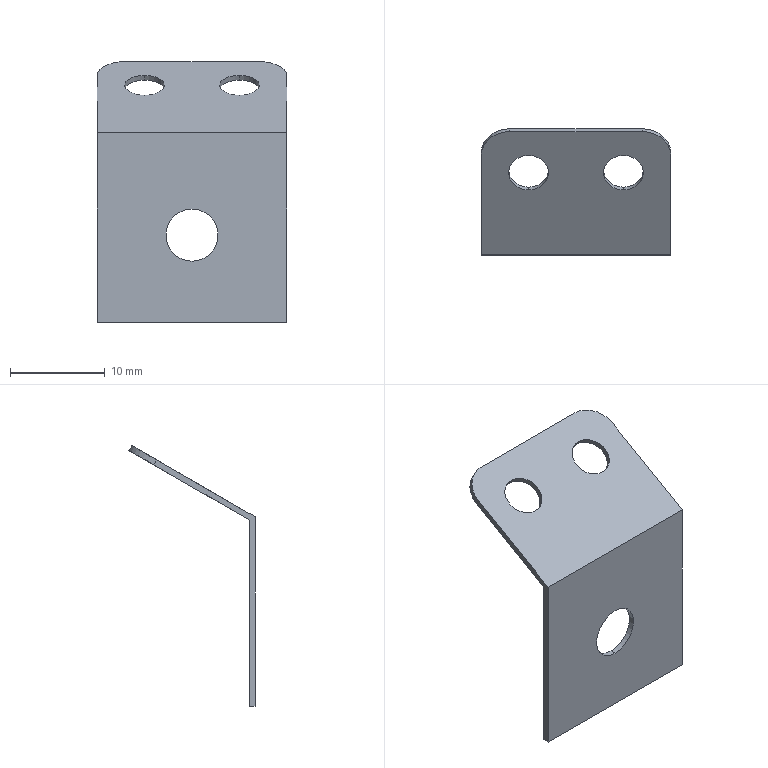Part | STEP file | Fiber fixing plate | 1 solid | 16 faces | box 20 x 13.29 x 27.5 mm | volume 382.645 mm3 | cylinder 8 | plane 8 | commonest cylinder face diameters 4.2 x4 5.5 x2 6 x2
STEP:
#1=CARTESIAN_POINT('',(0.,0.,0.));
#2=DIRECTION('',(0.,0.,1.));
#3=DIRECTION('',(1.,0.,0.));
#4=AXIS2_PLACEMENT_3D('',#1,#2,#3);
#5=CARTESIAN_POINT('',(15.,33.278,19.441));
#6=VERTEX_POINT('',#5);
#7=CARTESIAN_POINT('',(15.,32.978,19.96));
#8=VERTEX_POINT('',#7);
#9=CARTESIAN_POINT('',(15.,42.978,2.64));
#10=DIRECTION('',(0.,-0.5,0.866));
#11=VECTOR('',#10,1.);
#12=LINE('',#9,#11);
#13=CARTESIAN_POINT('',(15.,44.797,3.69));
#14=DIRECTION('',(0.,-0.5,0.866));
#15=DIRECTION('',(0.,-0.866,-0.5));
#16=AXIS2_PLACEMENT_3D('',#13,#14,#15);
#17=CYLINDRICAL_SURFACE('',#16,2.1);
#18=CARTESIAN_POINT('',(6.283,0.));
#19=DIRECTION('',(0.,1.));
#20=VECTOR('',#19,1.);
#21=LINE('',#18,#20);
#22=(GEOMETRIC_REPRESENTATION_CONTEXT(2)PARAMETRIC_REPRESENTATION_CONTEXT()REPRESENTATION_CONTEXT('',''));
#23=DEFINITIONAL_REPRESENTATION('',(#21),#22);
#24=PCURVE('',#17,#23);
#25=CARTESIAN_POINT('',(15.,44.797,3.69));
#26=DIRECTION('',(0.,-0.5,0.866));
#27=DIRECTION('',(0.,-0.866,-0.5));
#28=AXIS2_PLACEMENT_3D('',#25,#26,#27);
#29=CYLINDRICAL_SURFACE('',#28,2.1);
#30=CARTESIAN_POINT('',(0.,0.));
#31=DIRECTION('',(0.,1.));
#32=VECTOR('',#31,1.);
#33=LINE('',#30,#32);
#34=(GEOMETRIC_REPRESENTATION_CONTEXT(2)PARAMETRIC_REPRESENTATION_CONTEXT()REPRESENTATION_CONTEXT('',''));
#35=DEFINITIONAL_REPRESENTATION('',(#33),#34);
#36=PCURVE('',#29,#35);
#37=SURFACE_CURVE('',#12,(#24,#36),.PCURVE_S1.);
#38=EDGE_CURVE('',#6,#8,#37,.T.);
#39=ORIENTED_EDGE('',*,*,#38,.T.);
#40=CARTESIAN_POINT('',(15.,36.615,22.06));
#41=VERTEX_POINT('',#40);
#42=CARTESIAN_POINT('',(15.,34.797,21.01));
#43=DIRECTION('',(0.,-0.5,0.866));
#44=DIRECTION('',(0.,0.866,0.5));
#45=AXIS2_PLACEMENT_3D('',#42,#43,#44);
#46=CIRCLE('',#45,2.1);
#47=CARTESIAN_POINT('',(3.142,20.));
#48=DIRECTION('',(1.,0.));
#49=VECTOR('',#48,1.);
#50=LINE('',#47,#49);
#51=(GEOMETRIC_REPRESENTATION_CONTEXT(2)PARAMETRIC_REPRESENTATION_CONTEXT()REPRESENTATION_CONTEXT('',''));
#52=DEFINITIONAL_REPRESENTATION('',(#50),#51);
#53=PCURVE('',#17,#52);
#54=CARTESIAN_POINT('',(20.,26.136,16.01));
#55=DIRECTION('',(0.,0.5,-0.866));
#56=DIRECTION('',(0.,0.866,0.5));
#57=AXIS2_PLACEMENT_3D('',#54,#55,#56);
#58=PLANE('',#57);
#59=CARTESIAN_POINT('',(12.1,-5.));
#60=CARTESIAN_POINT('',(12.1,-8.637));
#61=CARTESIAN_POINT('',(8.95,-6.819));
#62=CARTESIAN_POINT('',(5.8,-5.));
#63=CARTESIAN_POINT('',(8.95,-3.181));
#64=CARTESIAN_POINT('',(12.1,-1.363));
#65=CARTESIAN_POINT('',(12.1,-5.));
#66=(BOUNDED_CURVE()B_SPLINE_CURVE(2,(#59,#60,#61,#62,#63,#64,#65),.UNSPECIFIED.,.T.,.F.)B_SPLINE_CURVE_WITH_KNOTS((1,2,2,2,2,1),(-2.094,0.,2.094,4.189,6.283,8.378),.UNSPECIFIED.)CURVE()GEOMETRIC_REPRESENTATION_ITEM()RATIONAL_B_SPLINE_CURVE((1.,0.5,1.,0.5,1.,0.5,1.))REPRESENTATION_ITEM(''));
#67=(GEOMETRIC_REPRESENTATION_CONTEXT(2)PARAMETRIC_REPRESENTATION_CONTEXT()REPRESENTATION_CONTEXT('',''));
#68=DEFINITIONAL_REPRESENTATION('',(#66),#67);
#69=PCURVE('',#58,#68);
#70=SURFACE_CURVE('',#46,(#53,#69),.PCURVE_S1.);
#71=EDGE_CURVE('',#41,#8,#70,.T.);
#72=ORIENTED_EDGE('',*,*,#71,.F.);
#73=CARTESIAN_POINT('',(15.,36.915,21.541));
#74=VERTEX_POINT('',#73);
#75=CARTESIAN_POINT('',(15.,46.615,4.74));
#76=DIRECTION('',(0.,-0.5,0.866));
#77=VECTOR('',#76,1.);
#78=LINE('',#75,#77);
#79=CARTESIAN_POINT('',(3.142,0.));
#80=DIRECTION('',(0.,1.));
#81=VECTOR('',#80,1.);
#82=LINE('',#79,#81);
#83=(GEOMETRIC_REPRESENTATION_CONTEXT(2)PARAMETRIC_REPRESENTATION_CONTEXT()REPRESENTATION_CONTEXT('',''));
#84=DEFINITIONAL_REPRESENTATION('',(#82),#83);
#85=PCURVE('',#17,#84);
#86=CARTESIAN_POINT('',(3.142,0.));
#87=DIRECTION('',(0.,1.));
#88=VECTOR('',#87,1.);
#89=LINE('',#86,#88);
#90=(GEOMETRIC_REPRESENTATION_CONTEXT(2)PARAMETRIC_REPRESENTATION_CONTEXT()REPRESENTATION_CONTEXT('',''));
#91=DEFINITIONAL_REPRESENTATION('',(#89),#90);
#92=PCURVE('',#29,#91);
#93=SURFACE_CURVE('',#78,(#85,#92),.PCURVE_S1.);
#94=EDGE_CURVE('',#74,#41,#93,.T.);
#95=ORIENTED_EDGE('',*,*,#94,.F.);
#96=CARTESIAN_POINT('',(15.,35.097,20.491));
#97=DIRECTION('',(0.,-0.5,0.866));
#98=DIRECTION('',(0.,-0.866,-0.5));
#99=AXIS2_PLACEMENT_3D('',#96,#97,#98);
#100=CIRCLE('',#99,2.1);
#101=CARTESIAN_POINT('',(0.,19.4));
#102=DIRECTION('',(1.,0.));
#103=VECTOR('',#102,1.);
#104=LINE('',#101,#103);
#105=(GEOMETRIC_REPRESENTATION_CONTEXT(2)PARAMETRIC_REPRESENTATION_CONTEXT()REPRESENTATION_CONTEXT('',''));
#106=DEFINITIONAL_REPRESENTATION('',(#104),#105);
#107=PCURVE('',#17,#106);
#108=CARTESIAN_POINT('',(20.,26.736,15.664));
#109=DIRECTION('',(0.,-0.5,0.866));
#110=DIRECTION('',(0.,-0.866,-0.5));
#111=AXIS2_PLACEMENT_3D('',#108,#109,#110);
#112=PLANE('',#111);
#113=CARTESIAN_POINT('',(-9.654,-5.));
#114=DIRECTION('',(1.,0.));
#115=AXIS2_PLACEMENT_2D('',#113,#114);
#116=CIRCLE('',#115,2.1);
#117=(GEOMETRIC_REPRESENTATION_CONTEXT(2)PARAMETRIC_REPRESENTATION_CONTEXT()REPRESENTATION_CONTEXT('',''));
#118=DEFINITIONAL_REPRESENTATION('',(#116),#117);
#119=PCURVE('',#112,#118);
#120=SURFACE_CURVE('',#100,(#107,#119),.PCURVE_S1.);
#121=EDGE_CURVE('',#74,#6,#120,.T.);
#122=ORIENTED_EDGE('',*,*,#121,.T.);
#123=EDGE_LOOP('',(#39,#72,#95,#122));
#124=FACE_BOUND('',#123,.F.);
#125=ADVANCED_FACE('',(#124),#17,.F.);
#126=CARTESIAN_POINT('',(5.,33.278,19.441));
#127=VERTEX_POINT('',#126);
#128=CARTESIAN_POINT('',(5.,32.978,19.96));
#129=VERTEX_POINT('',#128);
#130=CARTESIAN_POINT('',(5.,42.978,2.64));
#131=DIRECTION('',(0.,-0.5,0.866));
#132=VECTOR('',#131,1.);
#133=LINE('',#130,#132);
#134=CARTESIAN_POINT('',(5.,44.797,3.69));
#135=DIRECTION('',(0.,-0.5,0.866));
#136=DIRECTION('',(0.,-0.866,-0.5));
#137=AXIS2_PLACEMENT_3D('',#134,#135,#136);
#138=CYLINDRICAL_SURFACE('',#137,2.1);
#139=CARTESIAN_POINT('',(6.283,0.));
#140=DIRECTION('',(0.,1.));
#141=VECTOR('',#140,1.);
#142=LINE('',#139,#141);
#143=(GEOMETRIC_REPRESENTATION_CONTEXT(2)PARAMETRIC_REPRESENTATION_CONTEXT()REPRESENTATION_CONTEXT('',''));
#144=DEFINITIONAL_REPRESENTATION('',(#142),#143);
#145=PCURVE('',#138,#144);
#146=CARTESIAN_POINT('',(5.,44.797,3.69));
#147=DIRECTION('',(0.,-0.5,0.866));
#148=DIRECTION('',(0.,-0.866,-0.5));
#149=AXIS2_PLACEMENT_3D('',#146,#147,#148);
#150=CYLINDRICAL_SURFACE('',#149,2.1);
#151=CARTESIAN_POINT('',(0.,0.));
#152=DIRECTION('',(0.,1.));
#153=VECTOR('',#152,1.);
#154=LINE('',#151,#153);
#155=(GEOMETRIC_REPRESENTATION_CONTEXT(2)PARAMETRIC_REPRESENTATION_CONTEXT()REPRESENTATION_CONTEXT('',''));
#156=DEFINITIONAL_REPRESENTATION('',(#154),#155);
#157=PCURVE('',#150,#156);
#158=SURFACE_CURVE('',#133,(#145,#157),.PCURVE_S1.);
#159=EDGE_CURVE('',#127,#129,#158,.T.);
#160=ORIENTED_EDGE('',*,*,#159,.T.);
#161=CARTESIAN_POINT('',(5.,36.615,22.06));
#162=VERTEX_POINT('',#161);
#163=CARTESIAN_POINT('',(5.,34.797,21.01));
#164=DIRECTION('',(0.,-0.5,0.866));
#165=DIRECTION('',(0.,-0.866,-0.5));
#166=AXIS2_PLACEMENT_3D('',#163,#164,#165);
#167=CIRCLE('',#166,2.1);
#168=CARTESIAN_POINT('',(0.,20.));
#169=DIRECTION('',(1.,0.));
#170=VECTOR('',#169,1.);
#171=LINE('',#168,#170);
#172=(GEOMETRIC_REPRESENTATION_CONTEXT(2)PARAMETRIC_REPRESENTATION_CONTEXT()REPRESENTATION_CONTEXT('',''));
#173=DEFINITIONAL_REPRESENTATION('',(#171),#172);
#174=PCURVE('',#138,#173);
#175=CARTESIAN_POINT('',(7.9,-15.));
#176=CARTESIAN_POINT('',(7.9,-11.363));
#177=CARTESIAN_POINT('',(11.05,-13.181));
#178=CARTESIAN_POINT('',(14.2,-15.));
#179=CARTESIAN_POINT('',(11.05,-16.819));
#180=CARTESIAN_POINT('',(7.9,-18.637));
#181=CARTESIAN_POINT('',(7.9,-15.));
#182=(BOUNDED_CURVE()B_SPLINE_CURVE(2,(#175,#176,#177,#178,#179,#180,#181),.UNSPECIFIED.,.T.,.F.)B_SPLINE_CURVE_WITH_KNOTS((1,2,2,2,2,1),(-2.094,0.,2.094,4.189,6.283,8.378),.UNSPECIFIED.)CURVE()GEOMETRIC_REPRESENTATION_ITEM()RATIONAL_B_SPLINE_CURVE((1.,0.5,1.,0.5,1.,0.5,1.))REPRESENTATION_ITEM(''));
#183=(GEOMETRIC_REPRESENTATION_CONTEXT(2)PARAMETRIC_REPRESENTATION_CONTEXT()REPRESENTATION_CONTEXT('',''));
#184=DEFINITIONAL_REPRESENTATION('',(#182),#183);
#185=PCURVE('',#58,#184);
#186=SURFACE_CURVE('',#167,(#174,#185),.PCURVE_S1.);
#187=EDGE_CURVE('',#162,#129,#186,.T.);
#188=ORIENTED_EDGE('',*,*,#187,.F.);
#189=CARTESIAN_POINT('',(5.,36.915,21.541));
#190=VERTEX_POINT('',#189);
#191=CARTESIAN_POINT('',(5.,46.615,4.74));
#192=DIRECTION('',(0.,-0.5,0.866));
#193=VECTOR('',#192,1.);
#194=LINE('',#191,#193);
#195=CARTESIAN_POINT('',(3.142,0.));
#196=DIRECTION('',(0.,1.));
#197=VECTOR('',#196,1.);
#198=LINE('',#195,#197);
#199=(GEOMETRIC_REPRESENTATION_CONTEXT(2)PARAMETRIC_REPRESENTATION_CONTEXT()REPRESENTATION_CONTEXT('',''));
#200=DEFINITIONAL_REPRESENTATION('',(#198),#199);
#201=PCURVE('',#138,#200);
#202=CARTESIAN_POINT('',(3.142,0.));
#203=DIRECTION('',(0.,1.));
#204=VECTOR('',#203,1.);
#205=LINE('',#202,#204);
#206=(GEOMETRIC_REPRESENTATION_CONTEXT(2)PARAMETRIC_REPRESENTATION_CONTEXT()REPRESENTATION_CONTEXT('',''));
#207=DEFINITIONAL_REPRESENTATION('',(#205),#206);
#208=PCURVE('',#150,#207);
#209=SURFACE_CURVE('',#194,(#201,#208),.PCURVE_S1.);
#210=EDGE_CURVE('',#190,#162,#209,.T.);
#211=ORIENTED_EDGE('',*,*,#210,.F.);
#212=CARTESIAN_POINT('',(5.,35.097,20.491));
#213=DIRECTION('',(0.,-0.5,0.866));
#214=DIRECTION('',(0.,-0.866,-0.5));
#215=AXIS2_PLACEMENT_3D('',#212,#213,#214);
#216=CIRCLE('',#215,2.1);
#217=CARTESIAN_POINT('',(0.,19.4));
#218=DIRECTION('',(1.,0.));
#219=VECTOR('',#218,1.);
#220=LINE('',#217,#219);
#221=(GEOMETRIC_REPRESENTATION_CONTEXT(2)PARAMETRIC_REPRESENTATION_CONTEXT()REPRESENTATION_CONTEXT('',''));
#222=DEFINITIONAL_REPRESENTATION('',(#220),#221);
#223=PCURVE('',#138,#222);
#224=CARTESIAN_POINT('',(-9.654,-15.));
#225=DIRECTION('',(1.,0.));
#226=AXIS2_PLACEMENT_2D('',#224,#225);
#227=CIRCLE('',#226,2.1);
#228=(GEOMETRIC_REPRESENTATION_CONTEXT(2)PARAMETRIC_REPRESENTATION_CONTEXT()REPRESENTATION_CONTEXT('',''));
#229=DEFINITIONAL_REPRESENTATION('',(#227),#228);
#230=PCURVE('',#112,#229);
#231=SURFACE_CURVE('',#216,(#223,#230),.PCURVE_S1.);
#232=EDGE_CURVE('',#190,#127,#231,.T.);
#233=ORIENTED_EDGE('',*,*,#232,.T.);
#234=EDGE_LOOP('',(#160,#188,#211,#233));
#235=FACE_BOUND('',#234,.F.);
#236=ADVANCED_FACE('',(#235),#138,.F.);
#237=CARTESIAN_POINT('',(10.,26.136,7.965));
#238=VERTEX_POINT('',#237);
#239=CARTESIAN_POINT('',(10.,26.736,7.965));
#240=VERTEX_POINT('',#239);
#241=CARTESIAN_POINT('',(10.,6.736,7.965));
#242=DIRECTION('',(0.,1.,0.));
#243=VECTOR('',#242,1.);
#244=LINE('',#241,#243);
#245=CARTESIAN_POINT('',(10.,6.736,5.215));
#246=DIRECTION('',(0.,1.,0.));
#247=DIRECTION('',(0.,0.,1.));
#248=AXIS2_PLACEMENT_3D('',#245,#246,#247);
#249=CYLINDRICAL_SURFACE('',#248,2.75);
#250=CARTESIAN_POINT('',(6.283,0.));
#251=DIRECTION('',(0.,1.));
#252=VECTOR('',#251,1.);
#253=LINE('',#250,#252);
#254=(GEOMETRIC_REPRESENTATION_CONTEXT(2)PARAMETRIC_REPRESENTATION_CONTEXT()REPRESENTATION_CONTEXT('',''));
#255=DEFINITIONAL_REPRESENTATION('',(#253),#254);
#256=PCURVE('',#249,#255);
#257=CARTESIAN_POINT('',(10.,6.736,5.215));
#258=DIRECTION('',(0.,1.,0.));
#259=DIRECTION('',(0.,0.,1.));
#260=AXIS2_PLACEMENT_3D('',#257,#258,#259);
#261=CYLINDRICAL_SURFACE('',#260,2.75);
#262=CARTESIAN_POINT('',(0.,0.));
#263=DIRECTION('',(0.,1.));
#264=VECTOR('',#263,1.);
#265=LINE('',#262,#264);
#266=(GEOMETRIC_REPRESENTATION_CONTEXT(2)PARAMETRIC_REPRESENTATION_CONTEXT()REPRESENTATION_CONTEXT('',''));
#267=DEFINITIONAL_REPRESENTATION('',(#265),#266);
#268=PCURVE('',#261,#267);
#269=SURFACE_CURVE('',#244,(#256,#268),.PCURVE_S1.);
#270=EDGE_CURVE('',#238,#240,#269,.T.);
#271=ORIENTED_EDGE('',*,*,#270,.T.);
#272=CARTESIAN_POINT('',(10.,26.736,2.465));
#273=VERTEX_POINT('',#272);
#274=CARTESIAN_POINT('',(10.,26.736,5.215));
#275=DIRECTION('',(0.,1.,0.));
#276=DIRECTION('',(0.,0.,1.));
#277=AXIS2_PLACEMENT_3D('',#274,#275,#276);
#278=CIRCLE('',#277,2.75);
#279=CARTESIAN_POINT('',(0.,20.));
#280=DIRECTION('',(1.,0.));
#281=VECTOR('',#280,1.);
#282=LINE('',#279,#281);
#283=(GEOMETRIC_REPRESENTATION_CONTEXT(2)PARAMETRIC_REPRESENTATION_CONTEXT()REPRESENTATION_CONTEXT('',''));
#284=DEFINITIONAL_REPRESENTATION('',(#282),#283);
#285=PCURVE('',#249,#284);
#286=CARTESIAN_POINT('',(20.,26.736,-3.99));
#287=DIRECTION('',(0.,-1.,0.));
#288=DIRECTION('',(0.,0.,-1.));
#289=AXIS2_PLACEMENT_3D('',#286,#287,#288);
#290=PLANE('',#289);
#291=CARTESIAN_POINT('',(-11.955,-10.));
#292=CARTESIAN_POINT('',(-11.955,-5.237));
#293=CARTESIAN_POINT('',(-7.83,-7.618));
#294=CARTESIAN_POINT('',(-3.705,-10.));
#295=CARTESIAN_POINT('',(-7.83,-12.382));
#296=CARTESIAN_POINT('',(-11.955,-14.763));
#297=CARTESIAN_POINT('',(-11.955,-10.));
#298=(BOUNDED_CURVE()B_SPLINE_CURVE(2,(#291,#292,#293,#294,#295,#296,#297),.UNSPECIFIED.,.T.,.F.)B_SPLINE_CURVE_WITH_KNOTS((1,2,2,2,2,1),(-2.094,0.,2.094,4.189,6.283,8.378),.UNSPECIFIED.)CURVE()GEOMETRIC_REPRESENTATION_ITEM()RATIONAL_B_SPLINE_CURVE((1.,0.5,1.,0.5,1.,0.5,1.))REPRESENTATION_ITEM(''));
#299=(GEOMETRIC_REPRESENTATION_CONTEXT(2)PARAMETRIC_REPRESENTATION_CONTEXT()REPRESENTATION_CONTEXT('',''));
#300=DEFINITIONAL_REPRESENTATION('',(#298),#299);
#301=PCURVE('',#290,#300);
#302=SURFACE_CURVE('',#278,(#285,#301),.PCURVE_S1.);
#303=EDGE_CURVE('',#273,#240,#302,.T.);
#304=ORIENTED_EDGE('',*,*,#303,.F.);
#305=CARTESIAN_POINT('',(10.,26.136,2.465));
#306=VERTEX_POINT('',#305);
#307=CARTESIAN_POINT('',(10.,6.736,2.465));
#308=DIRECTION('',(0.,1.,0.));
#309=VECTOR('',#308,1.);
#310=LINE('',#307,#309);
#311=CARTESIAN_POINT('',(3.142,0.));
#312=DIRECTION('',(0.,1.));
#313=VECTOR('',#312,1.);
#314=LINE('',#311,#313);
#315=(GEOMETRIC_REPRESENTATION_CONTEXT(2)PARAMETRIC_REPRESENTATION_CONTEXT()REPRESENTATION_CONTEXT('',''));
#316=DEFINITIONAL_REPRESENTATION('',(#314),#315);
#317=PCURVE('',#249,#316);
#318=CARTESIAN_POINT('',(3.142,0.));
#319=DIRECTION('',(0.,1.));
#320=VECTOR('',#319,1.);
#321=LINE('',#318,#320);
#322=(GEOMETRIC_REPRESENTATION_CONTEXT(2)PARAMETRIC_REPRESENTATION_CONTEXT()REPRESENTATION_CONTEXT('',''));
#323=DEFINITIONAL_REPRESENTATION('',(#321),#322);
#324=PCURVE('',#261,#323);
#325=SURFACE_CURVE('',#310,(#317,#324),.PCURVE_S1.);
#326=EDGE_CURVE('',#306,#273,#325,.T.);
#327=ORIENTED_EDGE('',*,*,#326,.F.);
#328=CARTESIAN_POINT('',(10.,26.136,5.215));
#329=DIRECTION('',(0.,1.,0.));
#330=DIRECTION('',(0.,0.,1.));
#331=AXIS2_PLACEMENT_3D('',#328,#329,#330);
#332=CIRCLE('',#331,2.75);
#333=CARTESIAN_POINT('',(0.,19.4));
#334=DIRECTION('',(1.,0.));
#335=VECTOR('',#334,1.);
#336=LINE('',#333,#335);
#337=(GEOMETRIC_REPRESENTATION_CONTEXT(2)PARAMETRIC_REPRESENTATION_CONTEXT()REPRESENTATION_CONTEXT('',''));
#338=DEFINITIONAL_REPRESENTATION('',(#336),#337);
#339=PCURVE('',#249,#338);
#340=CARTESIAN_POINT('',(20.,26.136,-3.99));
#341=DIRECTION('',(0.,1.,0.));
#342=DIRECTION('',(0.,0.,1.));
#343=AXIS2_PLACEMENT_3D('',#340,#341,#342);
#344=PLANE('',#343);
#345=CARTESIAN_POINT('',(9.205,-10.));
#346=DIRECTION('',(1.,0.));
#347=AXIS2_PLACEMENT_2D('',#345,#346);
#348=CIRCLE('',#347,2.75);
#349=(GEOMETRIC_REPRESENTATION_CONTEXT(2)PARAMETRIC_REPRESENTATION_CONTEXT()REPRESENTATION_CONTEXT('',''));
#350=DEFINITIONAL_REPRESENTATION('',(#348),#349);
#351=PCURVE('',#344,#350);
#352=SURFACE_CURVE('',#332,(#339,#351),.PCURVE_S1.);
#353=EDGE_CURVE('',#306,#238,#352,.T.);
#354=ORIENTED_EDGE('',*,*,#353,.T.);
#355=EDGE_LOOP('',(#271,#304,#327,#354));
#356=FACE_BOUND('',#355,.F.);
#357=ADVANCED_FACE('',(#356),#249,.F.);
#358=CARTESIAN_POINT('',(0.,26.136,-3.99));
#359=VERTEX_POINT('',#358);
#360=CARTESIAN_POINT('',(0.,26.736,-3.99));
#361=VERTEX_POINT('',#360);
#362=CARTESIAN_POINT('',(0.,26.136,-3.99));
#363=DIRECTION('',(0.,1.,0.));
#364=VECTOR('',#363,1.);
#365=LINE('',#362,#364);
#366=CARTESIAN_POINT('',(20.,26.136,-3.99));
#367=DIRECTION('',(0.,0.,1.));
#368=DIRECTION('',(1.,0.,0.));
#369=AXIS2_PLACEMENT_3D('',#366,#367,#368);
#370=PLANE('',#369);
#371=CARTESIAN_POINT('',(-20.,0.));
#372=DIRECTION('',(0.,1.));
#373=VECTOR('',#372,1.);
#374=LINE('',#371,#373);
#375=(GEOMETRIC_REPRESENTATION_CONTEXT(2)PARAMETRIC_REPRESENTATION_CONTEXT()REPRESENTATION_CONTEXT('',''));
#376=DEFINITIONAL_REPRESENTATION('',(#374),#375);
#377=PCURVE('',#370,#376);
#378=CARTESIAN_POINT('',(0.,0.,0.));
#379=DIRECTION('',(1.,0.,0.));
#380=DIRECTION('',(0.,0.,-1.));
#381=AXIS2_PLACEMENT_3D('',#378,#379,#380);
#382=PLANE('',#381);
#383=CARTESIAN_POINT('',(3.99,26.136));
#384=DIRECTION('',(0.,1.));
#385=VECTOR('',#384,1.);
#386=LINE('',#383,#385);
#387=(GEOMETRIC_REPRESENTATION_CONTEXT(2)PARAMETRIC_REPRESENTATION_CONTEXT()REPRESENTATION_CONTEXT('',''));
#388=DEFINITIONAL_REPRESENTATION('',(#386),#387);
#389=PCURVE('',#382,#388);
#390=SURFACE_CURVE('',#365,(#377,#389),.PCURVE_S1.);
#391=EDGE_CURVE('',#359,#361,#390,.T.);
#392=ORIENTED_EDGE('',*,*,#391,.T.);
#393=CARTESIAN_POINT('',(20.,26.736,-3.99));
#394=VERTEX_POINT('',#393);
#395=CARTESIAN_POINT('',(20.,26.736,-3.99));
#396=DIRECTION('',(-1.,0.,0.));
#397=VECTOR('',#396,1.);
#398=LINE('',#395,#397);
#399=CARTESIAN_POINT('',(0.,0.6));
#400=DIRECTION('',(-1.,0.));
#401=VECTOR('',#400,1.);
#402=LINE('',#399,#401);
#403=(GEOMETRIC_REPRESENTATION_CONTEXT(2)PARAMETRIC_REPRESENTATION_CONTEXT()REPRESENTATION_CONTEXT('',''));
#404=DEFINITIONAL_REPRESENTATION('',(#402),#403);
#405=PCURVE('',#370,#404);
#406=CARTESIAN_POINT('',(0.,0.));
#407=DIRECTION('',(0.,-1.));
#408=VECTOR('',#407,1.);
#409=LINE('',#406,#408);
#410=(GEOMETRIC_REPRESENTATION_CONTEXT(2)PARAMETRIC_REPRESENTATION_CONTEXT()REPRESENTATION_CONTEXT('',''));
#411=DEFINITIONAL_REPRESENTATION('',(#409),#410);
#412=PCURVE('',#290,#411);
#413=SURFACE_CURVE('',#398,(#405,#412),.PCURVE_S1.);
#414=EDGE_CURVE('',#394,#361,#413,.T.);
#415=ORIENTED_EDGE('',*,*,#414,.F.);
#416=CARTESIAN_POINT('',(20.,26.136,-3.99));
#417=VERTEX_POINT('',#416);
#418=CARTESIAN_POINT('',(20.,26.136,-3.99));
#419=DIRECTION('',(0.,1.,0.));
#420=VECTOR('',#419,1.);
#421=LINE('',#418,#420);
#422=CARTESIAN_POINT('',(0.,0.));
#423=DIRECTION('',(0.,1.));
#424=VECTOR('',#423,1.);
#425=LINE('',#422,#424);
#426=(GEOMETRIC_REPRESENTATION_CONTEXT(2)PARAMETRIC_REPRESENTATION_CONTEXT()REPRESENTATION_CONTEXT('',''));
#427=DEFINITIONAL_REPRESENTATION('',(#425),#426);
#428=PCURVE('',#370,#427);
#429=CARTESIAN_POINT('',(20.,0.,0.));
#430=DIRECTION('',(1.,0.,0.));
#431=DIRECTION('',(0.,0.,-1.));
#432=AXIS2_PLACEMENT_3D('',#429,#430,#431);
#433=PLANE('',#432);
#434=CARTESIAN_POINT('',(3.99,26.136));
#435=DIRECTION('',(0.,1.));
#436=VECTOR('',#435,1.);
#437=LINE('',#434,#436);
#438=(GEOMETRIC_REPRESENTATION_CONTEXT(2)PARAMETRIC_REPRESENTATION_CONTEXT()REPRESENTATION_CONTEXT('',''));
#439=DEFINITIONAL_REPRESENTATION('',(#437),#438);
#440=PCURVE('',#433,#439);
#441=SURFACE_CURVE('',#421,(#428,#440),.PCURVE_S1.);
#442=EDGE_CURVE('',#417,#394,#441,.T.);
#443=ORIENTED_EDGE('',*,*,#442,.F.);
#444=CARTESIAN_POINT('',(20.,26.136,-3.99));
#445=DIRECTION('',(-1.,0.,0.));
#446=VECTOR('',#445,1.);
#447=LINE('',#444,#446);
#448=CARTESIAN_POINT('',(0.,0.));
#449=DIRECTION('',(-1.,0.));
#450=VECTOR('',#449,1.);
#451=LINE('',#448,#450);
#452=(GEOMETRIC_REPRESENTATION_CONTEXT(2)PARAMETRIC_REPRESENTATION_CONTEXT()REPRESENTATION_CONTEXT('',''));
#453=DEFINITIONAL_REPRESENTATION('',(#451),#452);
#454=PCURVE('',#370,#453);
#455=CARTESIAN_POINT('',(0.,0.));
#456=DIRECTION('',(0.,-1.));
#457=VECTOR('',#456,1.);
#458=LINE('',#455,#457);
#459=(GEOMETRIC_REPRESENTATION_CONTEXT(2)PARAMETRIC_REPRESENTATION_CONTEXT()REPRESENTATION_CONTEXT('',''));
#460=DEFINITIONAL_REPRESENTATION('',(#458),#459);
#461=PCURVE('',#344,#460);
#462=SURFACE_CURVE('',#447,(#454,#461),.PCURVE_S1.);
#463=EDGE_CURVE('',#417,#359,#462,.T.);
#464=ORIENTED_EDGE('',*,*,#463,.T.);
#465=EDGE_LOOP('',(#392,#415,#443,#464));
#466=FACE_BOUND('',#465,.T.);
#467=ADVANCED_FACE('',(#466),#370,.F.);
#468=CARTESIAN_POINT('',(10.,26.736,5.215));
#469=DIRECTION('',(0.,1.,0.));
#470=DIRECTION('',(0.,0.,1.));
#471=AXIS2_PLACEMENT_3D('',#468,#469,#470);
#472=CIRCLE('',#471,2.75);
#473=CARTESIAN_POINT('',(-11.955,-10.));
#474=CARTESIAN_POINT('',(-11.955,-5.237));
#475=CARTESIAN_POINT('',(-7.83,-7.618));
#476=CARTESIAN_POINT('',(-3.705,-10.));
#477=CARTESIAN_POINT('',(-7.83,-12.382));
#478=CARTESIAN_POINT('',(-11.955,-14.763));
#479=CARTESIAN_POINT('',(-11.955,-10.));
#480=(BOUNDED_CURVE()B_SPLINE_CURVE(2,(#473,#474,#475,#476,#477,#478,#479),.UNSPECIFIED.,.T.,.F.)B_SPLINE_CURVE_WITH_KNOTS((1,2,2,2,2,1),(-2.094,0.,2.094,4.189,6.283,8.378),.UNSPECIFIED.)CURVE()GEOMETRIC_REPRESENTATION_ITEM()RATIONAL_B_SPLINE_CURVE((1.,0.5,1.,0.5,1.,0.5,1.))REPRESENTATION_ITEM(''));
#481=(GEOMETRIC_REPRESENTATION_CONTEXT(2)PARAMETRIC_REPRESENTATION_CONTEXT()REPRESENTATION_CONTEXT('',''));
#482=DEFINITIONAL_REPRESENTATION('',(#480),#481);
#483=PCURVE('',#290,#482);
#484=CARTESIAN_POINT('',(0.,20.));
#485=DIRECTION('',(1.,0.));
#486=VECTOR('',#485,1.);
#487=LINE('',#484,#486);
#488=(GEOMETRIC_REPRESENTATION_CONTEXT(2)PARAMETRIC_REPRESENTATION_CONTEXT()REPRESENTATION_CONTEXT('',''));
#489=DEFINITIONAL_REPRESENTATION('',(#487),#488);
#490=PCURVE('',#261,#489);
#491=SURFACE_CURVE('',#472,(#483,#490),.PCURVE_S1.);
#492=EDGE_CURVE('',#240,#273,#491,.T.);
#493=ORIENTED_EDGE('',*,*,#492,.F.);
#494=ORIENTED_EDGE('',*,*,#303,.F.);
#495=EDGE_LOOP('',(#493,#494));
#496=FACE_BOUND('',#495,.T.);
#497=CARTESIAN_POINT('',(0.,26.736,15.664));
#498=VERTEX_POINT('',#497);
#499=CARTESIAN_POINT('',(0.,26.736,-3.99));
#500=DIRECTION('',(0.,0.,1.));
#501=VECTOR('',#500,1.);
#502=LINE('',#499,#501);
#503=CARTESIAN_POINT('',(0.,-20.));
#504=DIRECTION('',(-1.,0.));
#505=VECTOR('',#504,1.);
#506=LINE('',#503,#505);
#507=(GEOMETRIC_REPRESENTATION_CONTEXT(2)PARAMETRIC_REPRESENTATION_CONTEXT()REPRESENTATION_CONTEXT('',''));
#508=DEFINITIONAL_REPRESENTATION('',(#506),#507);
#509=PCURVE('',#290,#508);
#510=CARTESIAN_POINT('',(3.99,26.736));
#511=DIRECTION('',(-1.,0.));
#512=VECTOR('',#511,1.);
#513=LINE('',#510,#512);
#514=(GEOMETRIC_REPRESENTATION_CONTEXT(2)PARAMETRIC_REPRESENTATION_CONTEXT()REPRESENTATION_CONTEXT('',''));
#515=DEFINITIONAL_REPRESENTATION('',(#513),#514);
#516=PCURVE('',#382,#515);
#517=SURFACE_CURVE('',#502,(#509,#516),.PCURVE_S1.);
#518=EDGE_CURVE('',#361,#498,#517,.T.);
#519=ORIENTED_EDGE('',*,*,#518,.T.);
#520=CARTESIAN_POINT('',(20.,26.736,15.664));
#521=VERTEX_POINT('',#520);
#522=CARTESIAN_POINT('',(20.,26.736,15.664));
#523=DIRECTION('',(-1.,0.,0.));
#524=VECTOR('',#523,1.);
#525=LINE('',#522,#524);
#526=CARTESIAN_POINT('',(-19.654,0.));
#527=DIRECTION('',(0.,-1.));
#528=VECTOR('',#527,1.);
#529=LINE('',#526,#528);
#530=(GEOMETRIC_REPRESENTATION_CONTEXT(2)PARAMETRIC_REPRESENTATION_CONTEXT()REPRESENTATION_CONTEXT('',''));
#531=DEFINITIONAL_REPRESENTATION('',(#529),#530);
#532=PCURVE('',#290,#531);
#533=CARTESIAN_POINT('',(0.,0.));
#534=DIRECTION('',(0.,-1.));
#535=VECTOR('',#534,1.);
#536=LINE('',#533,#535);
#537=(GEOMETRIC_REPRESENTATION_CONTEXT(2)PARAMETRIC_REPRESENTATION_CONTEXT()REPRESENTATION_CONTEXT('',''));
#538=DEFINITIONAL_REPRESENTATION('',(#536),#537);
#539=PCURVE('',#112,#538);
#540=SURFACE_CURVE('',#525,(#532,#539),.PCURVE_S1.);
#541=EDGE_CURVE('',#521,#498,#540,.T.);
#542=ORIENTED_EDGE('',*,*,#541,.F.);
#543=CARTESIAN_POINT('',(20.,26.736,-3.99));
#544=DIRECTION('',(0.,0.,1.));
#545=VECTOR('',#544,1.);
#546=LINE('',#543,#545);
#547=CARTESIAN_POINT('',(0.,0.));
#548=DIRECTION('',(-1.,0.));
#549=VECTOR('',#548,1.);
#550=LINE('',#547,#549);
#551=(GEOMETRIC_REPRESENTATION_CONTEXT(2)PARAMETRIC_REPRESENTATION_CONTEXT()REPRESENTATION_CONTEXT('',''));
#552=DEFINITIONAL_REPRESENTATION('',(#550),#551);
#553=PCURVE('',#290,#552);
#554=CARTESIAN_POINT('',(3.99,26.736));
#555=DIRECTION('',(-1.,0.));
#556=VECTOR('',#555,1.);
#557=LINE('',#554,#556);
#558=(GEOMETRIC_REPRESENTATION_CONTEXT(2)PARAMETRIC_REPRESENTATION_CONTEXT()REPRESENTATION_CONTEXT('',''));
#559=DEFINITIONAL_REPRESENTATION('',(#557),#558);
#560=PCURVE('',#433,#559);
#561=SURFACE_CURVE('',#546,(#553,#560),.PCURVE_S1.);
#562=EDGE_CURVE('',#394,#521,#561,.T.);
#563=ORIENTED_EDGE('',*,*,#562,.F.);
#564=ORIENTED_EDGE('',*,*,#414,.T.);
#565=EDGE_LOOP('',(#519,#542,#563,#564));
#566=FACE_BOUND('',#565,.T.);
#567=ADVANCED_FACE('',(#496,#566),#290,.F.);
#568=CARTESIAN_POINT('',(15.,35.097,20.491));
#569=DIRECTION('',(0.,-0.5,0.866));
#570=DIRECTION('',(0.,-0.866,-0.5));
#571=AXIS2_PLACEMENT_3D('',#568,#569,#570);
#572=CIRCLE('',#571,2.1);
#573=CARTESIAN_POINT('',(-9.654,-5.));
#574=DIRECTION('',(1.,0.));
#575=AXIS2_PLACEMENT_2D('',#573,#574);
#576=CIRCLE('',#575,2.1);
#577=(GEOMETRIC_REPRESENTATION_CONTEXT(2)PARAMETRIC_REPRESENTATION_CONTEXT()REPRESENTATION_CONTEXT('',''));
#578=DEFINITIONAL_REPRESENTATION('',(#576),#577);
#579=PCURVE('',#112,#578);
#580=CARTESIAN_POINT('',(0.,19.4));
#581=DIRECTION('',(1.,0.));
#582=VECTOR('',#581,1.);
#583=LINE('',#580,#582);
#584=(GEOMETRIC_REPRESENTATION_CONTEXT(2)PARAMETRIC_REPRESENTATION_CONTEXT()REPRESENTATION_CONTEXT('',''));
#585=DEFINITIONAL_REPRESENTATION('',(#583),#584);
#586=PCURVE('',#29,#585);
#587=SURFACE_CURVE('',#572,(#579,#586),.PCURVE_S1.);
#588=EDGE_CURVE('',#6,#74,#587,.T.);
#589=ORIENTED_EDGE('',*,*,#588,.T.);
#590=ORIENTED_EDGE('',*,*,#121,.T.);
#591=EDGE_LOOP('',(#589,#590));
#592=FACE_BOUND('',#591,.T.);
#593=CARTESIAN_POINT('',(5.,35.097,20.491));
#594=DIRECTION('',(0.,-0.5,0.866));
#595=DIRECTION('',(0.,-0.866,-0.5));
#596=AXIS2_PLACEMENT_3D('',#593,#594,#595);
#597=CIRCLE('',#596,2.1);
#598=CARTESIAN_POINT('',(-9.654,-15.));
#599=DIRECTION('',(1.,0.));
#600=AXIS2_PLACEMENT_2D('',#598,#599);
#601=CIRCLE('',#600,2.1);
#602=(GEOMETRIC_REPRESENTATION_CONTEXT(2)PARAMETRIC_REPRESENTATION_CONTEXT()REPRESENTATION_CONTEXT('',''));
#603=DEFINITIONAL_REPRESENTATION('',(#601),#602);
#604=PCURVE('',#112,#603);
#605=CARTESIAN_POINT('',(0.,19.4));
#606=DIRECTION('',(1.,0.));
#607=VECTOR('',#606,1.);
#608=LINE('',#605,#607);
#609=(GEOMETRIC_REPRESENTATION_CONTEXT(2)PARAMETRIC_REPRESENTATION_CONTEXT()REPRESENTATION_CONTEXT('',''));
#610=DEFINITIONAL_REPRESENTATION('',(#608),#609);
#611=PCURVE('',#150,#610);
#612=SURFACE_CURVE('',#597,(#604,#611),.PCURVE_S1.);
#613=EDGE_CURVE('',#127,#190,#612,.T.);
#614=ORIENTED_EDGE('',*,*,#613,.T.);
#615=ORIENTED_EDGE('',*,*,#232,.T.);
#616=EDGE_LOOP('',(#614,#615));
#617=FACE_BOUND('',#616,.T.);
#618=CARTESIAN_POINT('',(17.,39.427,22.991));
#619=VERTEX_POINT('',#618);
#620=CARTESIAN_POINT('',(3.,39.427,22.991));
#621=VERTEX_POINT('',#620);
#622=CARTESIAN_POINT('',(20.,39.427,22.991));
#623=DIRECTION('',(-1.,0.,0.));
#624=VECTOR('',#623,1.);
#625=LINE('',#622,#624);
#626=CARTESIAN_POINT('',(-14.654,0.));
#627=DIRECTION('',(0.,-1.));
#628=VECTOR('',#627,1.);
#629=LINE('',#626,#628);
#630=(GEOMETRIC_REPRESENTATION_CONTEXT(2)PARAMETRIC_REPRESENTATION_CONTEXT()REPRESENTATION_CONTEXT('',''));
#631=DEFINITIONAL_REPRESENTATION('',(#629),#630);
#632=PCURVE('',#112,#631);
#633=CARTESIAN_POINT('',(20.,39.127,23.51));
#634=DIRECTION('',(0.,-0.866,-0.5));
#635=DIRECTION('',(0.,0.5,-0.866));
#636=AXIS2_PLACEMENT_3D('',#633,#634,#635);
#637=PLANE('',#636);
#638=CARTESIAN_POINT('',(0.6,0.));
#639=DIRECTION('',(0.,-1.));
#640=VECTOR('',#639,1.);
#641=LINE('',#638,#640);
#642=(GEOMETRIC_REPRESENTATION_CONTEXT(2)PARAMETRIC_REPRESENTATION_CONTEXT()REPRESENTATION_CONTEXT('',''));
#643=DEFINITIONAL_REPRESENTATION('',(#641),#642);
#644=PCURVE('',#637,#643);
#645=SURFACE_CURVE('',#625,(#632,#644),.PCURVE_S1.);
#646=EDGE_CURVE('',#619,#621,#645,.T.);
#647=ORIENTED_EDGE('',*,*,#646,.F.);
#648=CARTESIAN_POINT('',(20.,36.829,21.491));
#649=VERTEX_POINT('',#648);
#650=CARTESIAN_POINT('',(17.,36.829,21.491));
#651=DIRECTION('',(0.,0.5,-0.866));
#652=DIRECTION('',(0.,-0.866,-0.5));
#653=AXIS2_PLACEMENT_3D('',#650,#651,#652);
#654=CIRCLE('',#653,3.);
#655=CARTESIAN_POINT('',(-8.654,-3.));
#656=CARTESIAN_POINT('',(-8.654,-8.196));
#657=CARTESIAN_POINT('',(-13.154,-5.598));
#658=CARTESIAN_POINT('',(-17.654,-3.));
#659=CARTESIAN_POINT('',(-13.154,-0.4019));
#660=CARTESIAN_POINT('',(-8.654,2.196));
#661=CARTESIAN_POINT('',(-8.654,-3.));
#662=(BOUNDED_CURVE()B_SPLINE_CURVE(2,(#655,#656,#657,#658,#659,#660,#661),.UNSPECIFIED.,.T.,.F.)B_SPLINE_CURVE_WITH_KNOTS((1,2,2,2,2,1),(-2.094,0.,2.094,4.189,6.283,8.378),.UNSPECIFIED.)CURVE()GEOMETRIC_REPRESENTATION_ITEM()RATIONAL_B_SPLINE_CURVE((1.,0.5,1.,0.5,1.,0.5,1.))REPRESENTATION_ITEM(''));
#663=(GEOMETRIC_REPRESENTATION_CONTEXT(2)PARAMETRIC_REPRESENTATION_CONTEXT()REPRESENTATION_CONTEXT('',''));
#664=DEFINITIONAL_REPRESENTATION('',(#662),#663);
#665=PCURVE('',#112,#664);
#666=CARTESIAN_POINT('',(17.,36.927,21.32));
#667=DIRECTION('',(0.,0.5,-0.866));
#668=DIRECTION('',(0.,0.866,0.5));
#669=AXIS2_PLACEMENT_3D('',#666,#667,#668);
#670=CYLINDRICAL_SURFACE('',#669,3.);
#671=CARTESIAN_POINT('',(-3.142,-0.1971));
#672=DIRECTION('',(1.,0.));
#673=VECTOR('',#672,1.);
#674=LINE('',#671,#673);
#675=(GEOMETRIC_REPRESENTATION_CONTEXT(2)PARAMETRIC_REPRESENTATION_CONTEXT()REPRESENTATION_CONTEXT('',''));
#676=DEFINITIONAL_REPRESENTATION('',(#674),#675);
#677=PCURVE('',#670,#676);
#678=SURFACE_CURVE('',#654,(#665,#677),.PCURVE_S1.);
#679=EDGE_CURVE('',#619,#649,#678,.T.);
#680=ORIENTED_EDGE('',*,*,#679,.T.);
#681=CARTESIAN_POINT('',(20.,26.736,15.664));
#682=DIRECTION('',(0.,0.866,0.5));
#683=VECTOR('',#682,1.);
#684=LINE('',#681,#683);
#685=CARTESIAN_POINT('',(0.,0.));
#686=DIRECTION('',(-1.,0.));
#687=VECTOR('',#686,1.);
#688=LINE('',#685,#687);
#689=(GEOMETRIC_REPRESENTATION_CONTEXT(2)PARAMETRIC_REPRESENTATION_CONTEXT()REPRESENTATION_CONTEXT('',''));
#690=DEFINITIONAL_REPRESENTATION('',(#688),#689);
#691=PCURVE('',#112,#690);
#692=CARTESIAN_POINT('',(-15.664,26.736));
#693=DIRECTION('',(-0.5,0.866));
#694=VECTOR('',#693,1.);
#695=LINE('',#692,#694);
#696=(GEOMETRIC_REPRESENTATION_CONTEXT(2)PARAMETRIC_REPRESENTATION_CONTEXT()REPRESENTATION_CONTEXT('',''));
#697=DEFINITIONAL_REPRESENTATION('',(#695),#696);
#698=PCURVE('',#433,#697);
#699=SURFACE_CURVE('',#684,(#691,#698),.PCURVE_S1.);
#700=EDGE_CURVE('',#521,#649,#699,.T.);
#701=ORIENTED_EDGE('',*,*,#700,.F.);
#702=ORIENTED_EDGE('',*,*,#541,.T.);
#703=CARTESIAN_POINT('',(0.,36.829,21.491));
#704=VERTEX_POINT('',#703);
#705=CARTESIAN_POINT('',(0.,26.736,15.664));
#706=DIRECTION('',(0.,0.866,0.5));
#707=VECTOR('',#706,1.);
#708=LINE('',#705,#707);
#709=CARTESIAN_POINT('',(0.,-20.));
#710=DIRECTION('',(-1.,0.));
#711=VECTOR('',#710,1.);
#712=LINE('',#709,#711);
#713=(GEOMETRIC_REPRESENTATION_CONTEXT(2)PARAMETRIC_REPRESENTATION_CONTEXT()REPRESENTATION_CONTEXT('',''));
#714=DEFINITIONAL_REPRESENTATION('',(#712),#713);
#715=PCURVE('',#112,#714);
#716=CARTESIAN_POINT('',(-15.664,26.736));
#717=DIRECTION('',(-0.5,0.866));
#718=VECTOR('',#717,1.);
#719=LINE('',#716,#718);
#720=(GEOMETRIC_REPRESENTATION_CONTEXT(2)PARAMETRIC_REPRESENTATION_CONTEXT()REPRESENTATION_CONTEXT('',''));
#721=DEFINITIONAL_REPRESENTATION('',(#719),#720);
#722=PCURVE('',#382,#721);
#723=SURFACE_CURVE('',#708,(#715,#722),.PCURVE_S1.);
#724=EDGE_CURVE('',#498,#704,#723,.T.);
#725=ORIENTED_EDGE('',*,*,#724,.T.);
#726=CARTESIAN_POINT('',(3.,36.829,21.491));
#727=DIRECTION('',(0.,0.5,-0.866));
#728=DIRECTION('',(0.,-0.866,-0.5));
#729=AXIS2_PLACEMENT_3D('',#726,#727,#728);
#730=CIRCLE('',#729,3.);
#731=CARTESIAN_POINT('',(-8.654,-17.));
#732=CARTESIAN_POINT('',(-8.654,-22.196));
#733=CARTESIAN_POINT('',(-13.154,-19.598));
#734=CARTESIAN_POINT('',(-17.654,-17.));
#735=CARTESIAN_POINT('',(-13.154,-14.402));
#736=CARTESIAN_POINT('',(-8.654,-11.804));
#737=CARTESIAN_POINT('',(-8.654,-17.));
#738=(BOUNDED_CURVE()B_SPLINE_CURVE(2,(#731,#732,#733,#734,#735,#736,#737),.UNSPECIFIED.,.T.,.F.)B_SPLINE_CURVE_WITH_KNOTS((1,2,2,2,2,1),(-2.094,0.,2.094,4.189,6.283,8.378),.UNSPECIFIED.)CURVE()GEOMETRIC_REPRESENTATION_ITEM()RATIONAL_B_SPLINE_CURVE((1.,0.5,1.,0.5,1.,0.5,1.))REPRESENTATION_ITEM(''));
#739=(GEOMETRIC_REPRESENTATION_CONTEXT(2)PARAMETRIC_REPRESENTATION_CONTEXT()REPRESENTATION_CONTEXT('',''));
#740=DEFINITIONAL_REPRESENTATION('',(#738),#739);
#741=PCURVE('',#112,#740);
#742=CARTESIAN_POINT('',(3.,36.529,22.01));
#743=DIRECTION('',(0.,-0.5,0.866));
#744=DIRECTION('',(0.,-0.866,-0.5));
#745=AXIS2_PLACEMENT_3D('',#742,#743,#744);
#746=CYLINDRICAL_SURFACE('',#745,3.);
#747=CARTESIAN_POINT('',(6.283,-0.6));
#748=DIRECTION('',(-1.,0.));
#749=VECTOR('',#748,1.);
#750=LINE('',#747,#749);
#751=(GEOMETRIC_REPRESENTATION_CONTEXT(2)PARAMETRIC_REPRESENTATION_CONTEXT()REPRESENTATION_CONTEXT('',''));
#752=DEFINITIONAL_REPRESENTATION('',(#750),#751);
#753=PCURVE('',#746,#752);
#754=SURFACE_CURVE('',#730,(#741,#753),.PCURVE_S1.);
#755=EDGE_CURVE('',#704,#621,#754,.T.);
#756=ORIENTED_EDGE('',*,*,#755,.T.);
#757=EDGE_LOOP('',(#647,#680,#701,#702,#725,#756));
#758=FACE_BOUND('',#757,.T.);
#759=ADVANCED_FACE('',(#592,#617,#758),#112,.F.);
#760=CARTESIAN_POINT('',(17.,39.127,23.51));
#761=VERTEX_POINT('',#760);
#762=CARTESIAN_POINT('',(3.,39.127,23.51));
#763=VERTEX_POINT('',#762);
#764=CARTESIAN_POINT('',(20.,39.127,23.51));
#765=DIRECTION('',(-1.,0.,0.));
#766=VECTOR('',#765,1.);
#767=LINE('',#764,#766);
#768=CARTESIAN_POINT('',(0.,0.));
#769=DIRECTION('',(0.,-1.));
#770=VECTOR('',#769,1.);
#771=LINE('',#768,#770);
#772=(GEOMETRIC_REPRESENTATION_CONTEXT(2)PARAMETRIC_REPRESENTATION_CONTEXT()REPRESENTATION_CONTEXT('',''));
#773=DEFINITIONAL_REPRESENTATION('',(#771),#772);
#774=PCURVE('',#637,#773);
#775=CARTESIAN_POINT('',(15.,0.));
#776=DIRECTION('',(0.,-1.));
#777=VECTOR('',#776,1.);
#778=LINE('',#775,#777);
#779=(GEOMETRIC_REPRESENTATION_CONTEXT(2)PARAMETRIC_REPRESENTATION_CONTEXT()REPRESENTATION_CONTEXT('',''));
#780=DEFINITIONAL_REPRESENTATION('',(#778),#779);
#781=PCURVE('',#58,#780);
#782=SURFACE_CURVE('',#767,(#774,#781),.PCURVE_S1.);
#783=EDGE_CURVE('',#761,#763,#782,.T.);
#784=ORIENTED_EDGE('',*,*,#783,.F.);
#785=CARTESIAN_POINT('',(17.,39.427,22.991));
#786=DIRECTION('',(0.,0.5,-0.866));
#787=VECTOR('',#786,1.);
#788=LINE('',#785,#787);
#789=CARTESIAN_POINT('',(0.6,-3.));
#790=DIRECTION('',(1.,0.));
#791=VECTOR('',#790,1.);
#792=LINE('',#789,#791);
#793=(GEOMETRIC_REPRESENTATION_CONTEXT(2)PARAMETRIC_REPRESENTATION_CONTEXT()REPRESENTATION_CONTEXT('',''));
#794=DEFINITIONAL_REPRESENTATION('',(#792),#793);
#795=PCURVE('',#637,#794);
#796=CARTESIAN_POINT('',(0.,-0.1971));
#797=DIRECTION('',(0.,1.));
#798=VECTOR('',#797,1.);
#799=LINE('',#796,#798);
#800=(GEOMETRIC_REPRESENTATION_CONTEXT(2)PARAMETRIC_REPRESENTATION_CONTEXT()REPRESENTATION_CONTEXT('',''));
#801=DEFINITIONAL_REPRESENTATION('',(#799),#800);
#802=PCURVE('',#670,#801);
#803=SURFACE_CURVE('',#788,(#795,#802),.PCURVE_S1.);
#804=EDGE_CURVE('',#761,#619,#803,.T.);
#805=ORIENTED_EDGE('',*,*,#804,.T.);
#806=ORIENTED_EDGE('',*,*,#646,.T.);
#807=CARTESIAN_POINT('',(3.,39.127,23.51));
#808=DIRECTION('',(0.,-0.5,0.866));
#809=VECTOR('',#808,1.);
#810=LINE('',#807,#809);
#811=CARTESIAN_POINT('',(0.,-17.));
#812=DIRECTION('',(-1.,0.));
#813=VECTOR('',#812,1.);
#814=LINE('',#811,#813);
#815=(GEOMETRIC_REPRESENTATION_CONTEXT(2)PARAMETRIC_REPRESENTATION_CONTEXT()REPRESENTATION_CONTEXT('',''));
#816=DEFINITIONAL_REPRESENTATION('',(#814),#815);
#817=PCURVE('',#637,#816);
#818=CARTESIAN_POINT('',(3.142,0.));
#819=DIRECTION('',(0.,1.));
#820=VECTOR('',#819,1.);
#821=LINE('',#818,#820);
#822=(GEOMETRIC_REPRESENTATION_CONTEXT(2)PARAMETRIC_REPRESENTATION_CONTEXT()REPRESENTATION_CONTEXT('',''));
#823=DEFINITIONAL_REPRESENTATION('',(#821),#822);
#824=PCURVE('',#746,#823);
#825=SURFACE_CURVE('',#810,(#817,#824),.PCURVE_S1.);
#826=EDGE_CURVE('',#621,#763,#825,.T.);
#827=ORIENTED_EDGE('',*,*,#826,.T.);
#828=EDGE_LOOP('',(#784,#805,#806,#827));
#829=FACE_BOUND('',#828,.T.);
#830=ADVANCED_FACE('',(#829),#637,.F.);
#831=CARTESIAN_POINT('',(15.,34.797,21.01));
#832=DIRECTION('',(0.,-0.5,0.866));
#833=DIRECTION('',(0.,0.866,0.5));
#834=AXIS2_PLACEMENT_3D('',#831,#832,#833);
#835=CIRCLE('',#834,2.1);
#836=CARTESIAN_POINT('',(12.1,-5.));
#837=CARTESIAN_POINT('',(12.1,-8.637));
#838=CARTESIAN_POINT('',(8.95,-6.819));
#839=CARTESIAN_POINT('',(5.8,-5.));
#840=CARTESIAN_POINT('',(8.95,-3.181));
#841=CARTESIAN_POINT('',(12.1,-1.363));
#842=CARTESIAN_POINT('',(12.1,-5.));
#843=(BOUNDED_CURVE()B_SPLINE_CURVE(2,(#836,#837,#838,#839,#840,#841,#842),.UNSPECIFIED.,.T.,.F.)B_SPLINE_CURVE_WITH_KNOTS((1,2,2,2,2,1),(-2.094,0.,2.094,4.189,6.283,8.378),.UNSPECIFIED.)CURVE()GEOMETRIC_REPRESENTATION_ITEM()RATIONAL_B_SPLINE_CURVE((1.,0.5,1.,0.5,1.,0.5,1.))REPRESENTATION_ITEM(''));
#844=(GEOMETRIC_REPRESENTATION_CONTEXT(2)PARAMETRIC_REPRESENTATION_CONTEXT()REPRESENTATION_CONTEXT('',''));
#845=DEFINITIONAL_REPRESENTATION('',(#843),#844);
#846=PCURVE('',#58,#845);
#847=CARTESIAN_POINT('',(-3.142,20.));
#848=DIRECTION('',(1.,0.));
#849=VECTOR('',#848,1.);
#850=LINE('',#847,#849);
#851=(GEOMETRIC_REPRESENTATION_CONTEXT(2)PARAMETRIC_REPRESENTATION_CONTEXT()REPRESENTATION_CONTEXT('',''));
#852=DEFINITIONAL_REPRESENTATION('',(#850),#851);
#853=PCURVE('',#29,#852);
#854=SURFACE_CURVE('',#835,(#846,#853),.PCURVE_S1.);
#855=EDGE_CURVE('',#8,#41,#854,.T.);
#856=ORIENTED_EDGE('',*,*,#855,.F.);
#857=ORIENTED_EDGE('',*,*,#71,.F.);
#858=EDGE_LOOP('',(#856,#857));
#859=FACE_BOUND('',#858,.T.);
#860=CARTESIAN_POINT('',(5.,34.797,21.01));
#861=DIRECTION('',(0.,-0.5,0.866));
#862=DIRECTION('',(0.,-0.866,-0.5));
#863=AXIS2_PLACEMENT_3D('',#860,#861,#862);
#864=CIRCLE('',#863,2.1);
#865=CARTESIAN_POINT('',(7.9,-15.));
#866=CARTESIAN_POINT('',(7.9,-11.363));
#867=CARTESIAN_POINT('',(11.05,-13.181));
#868=CARTESIAN_POINT('',(14.2,-15.));
#869=CARTESIAN_POINT('',(11.05,-16.819));
#870=CARTESIAN_POINT('',(7.9,-18.637));
#871=CARTESIAN_POINT('',(7.9,-15.));
#872=(BOUNDED_CURVE()B_SPLINE_CURVE(2,(#865,#866,#867,#868,#869,#870,#871),.UNSPECIFIED.,.T.,.F.)B_SPLINE_CURVE_WITH_KNOTS((1,2,2,2,2,1),(-2.094,0.,2.094,4.189,6.283,8.378),.UNSPECIFIED.)CURVE()GEOMETRIC_REPRESENTATION_ITEM()RATIONAL_B_SPLINE_CURVE((1.,0.5,1.,0.5,1.,0.5,1.))REPRESENTATION_ITEM(''));
#873=(GEOMETRIC_REPRESENTATION_CONTEXT(2)PARAMETRIC_REPRESENTATION_CONTEXT()REPRESENTATION_CONTEXT('',''));
#874=DEFINITIONAL_REPRESENTATION('',(#872),#873);
#875=PCURVE('',#58,#874);
#876=CARTESIAN_POINT('',(0.,20.));
#877=DIRECTION('',(1.,0.));
#878=VECTOR('',#877,1.);
#879=LINE('',#876,#878);
#880=(GEOMETRIC_REPRESENTATION_CONTEXT(2)PARAMETRIC_REPRESENTATION_CONTEXT()REPRESENTATION_CONTEXT('',''));
#881=DEFINITIONAL_REPRESENTATION('',(#879),#880);
#882=PCURVE('',#150,#881);
#883=SURFACE_CURVE('',#864,(#875,#882),.PCURVE_S1.);
#884=EDGE_CURVE('',#129,#162,#883,.T.);
#885=ORIENTED_EDGE('',*,*,#884,.F.);
#886=ORIENTED_EDGE('',*,*,#187,.F.);
#887=EDGE_LOOP('',(#885,#886));
#888=FACE_BOUND('',#887,.T.);
#889=CARTESIAN_POINT('',(20.,36.529,22.01));
#890=VERTEX_POINT('',#889);
#891=CARTESIAN_POINT('',(20.,26.136,16.01));
#892=VERTEX_POINT('',#891);
#893=CARTESIAN_POINT('',(20.,26.136,16.01));
#894=DIRECTION('',(0.,-0.866,-0.5));
#895=VECTOR('',#894,1.);
#896=LINE('',#893,#895);
#897=CARTESIAN_POINT('',(0.,0.));
#898=DIRECTION('',(-1.,0.));
#899=VECTOR('',#898,1.);
#900=LINE('',#897,#899);
#901=(GEOMETRIC_REPRESENTATION_CONTEXT(2)PARAMETRIC_REPRESENTATION_CONTEXT()REPRESENTATION_CONTEXT('',''));
#902=DEFINITIONAL_REPRESENTATION('',(#900),#901);
#903=PCURVE('',#58,#902);
#904=CARTESIAN_POINT('',(-16.01,26.136));
#905=DIRECTION('',(0.5,-0.866));
#906=VECTOR('',#905,1.);
#907=LINE('',#904,#906);
#908=(GEOMETRIC_REPRESENTATION_CONTEXT(2)PARAMETRIC_REPRESENTATION_CONTEXT()REPRESENTATION_CONTEXT('',''));
#909=DEFINITIONAL_REPRESENTATION('',(#907),#908);
#910=PCURVE('',#433,#909);
#911=SURFACE_CURVE('',#896,(#903,#910),.PCURVE_S1.);
#912=EDGE_CURVE('',#890,#892,#911,.T.);
#913=ORIENTED_EDGE('',*,*,#912,.F.);
#914=CARTESIAN_POINT('',(17.,36.529,22.01));
#915=DIRECTION('',(0.,-0.5,0.866));
#916=DIRECTION('',(0.,0.866,0.5));
#917=AXIS2_PLACEMENT_3D('',#914,#915,#916);
#918=CIRCLE('',#917,3.);
#919=CARTESIAN_POINT('',(15.,-3.));
#920=CARTESIAN_POINT('',(15.,-8.196));
#921=CARTESIAN_POINT('',(10.5,-5.598));
#922=CARTESIAN_POINT('',(6.,-3.));
#923=CARTESIAN_POINT('',(10.5,-0.4019));
#924=CARTESIAN_POINT('',(15.,2.196));
#925=CARTESIAN_POINT('',(15.,-3.));
#926=(BOUNDED_CURVE()B_SPLINE_CURVE(2,(#919,#920,#921,#922,#923,#924,#925),.UNSPECIFIED.,.T.,.F.)B_SPLINE_CURVE_WITH_KNOTS((1,2,2,2,2,1),(-2.094,0.,2.094,4.189,6.283,8.378),.UNSPECIFIED.)CURVE()GEOMETRIC_REPRESENTATION_ITEM()RATIONAL_B_SPLINE_CURVE((1.,0.5,1.,0.5,1.,0.5,1.))REPRESENTATION_ITEM(''));
#927=(GEOMETRIC_REPRESENTATION_CONTEXT(2)PARAMETRIC_REPRESENTATION_CONTEXT()REPRESENTATION_CONTEXT('',''));
#928=DEFINITIONAL_REPRESENTATION('',(#926),#927);
#929=PCURVE('',#58,#928);
#930=CARTESIAN_POINT('',(6.283,-0.7971));
#931=DIRECTION('',(-1.,0.));
#932=VECTOR('',#931,1.);
#933=LINE('',#930,#932);
#934=(GEOMETRIC_REPRESENTATION_CONTEXT(2)PARAMETRIC_REPRESENTATION_CONTEXT()REPRESENTATION_CONTEXT('',''));
#935=DEFINITIONAL_REPRESENTATION('',(#933),#934);
#936=PCURVE('',#670,#935);
#937=SURFACE_CURVE('',#918,(#929,#936),.PCURVE_S1.);
#938=EDGE_CURVE('',#890,#761,#937,.T.);
#939=ORIENTED_EDGE('',*,*,#938,.T.);
#940=ORIENTED_EDGE('',*,*,#783,.T.);
#941=CARTESIAN_POINT('',(0.,36.529,22.01));
#942=VERTEX_POINT('',#941);
#943=CARTESIAN_POINT('',(3.,36.529,22.01));
#944=DIRECTION('',(0.,-0.5,0.866));
#945=DIRECTION('',(0.,0.866,0.5));
#946=AXIS2_PLACEMENT_3D('',#943,#944,#945);
#947=CIRCLE('',#946,3.);
#948=CARTESIAN_POINT('',(15.,-17.));
#949=CARTESIAN_POINT('',(15.,-22.196));
#950=CARTESIAN_POINT('',(10.5,-19.598));
#951=CARTESIAN_POINT('',(6.,-17.));
#952=CARTESIAN_POINT('',(10.5,-14.402));
#953=CARTESIAN_POINT('',(15.,-11.804));
#954=CARTESIAN_POINT('',(15.,-17.));
#955=(BOUNDED_CURVE()B_SPLINE_CURVE(2,(#948,#949,#950,#951,#952,#953,#954),.UNSPECIFIED.,.T.,.F.)B_SPLINE_CURVE_WITH_KNOTS((1,2,2,2,2,1),(-2.094,0.,2.094,4.189,6.283,8.378),.UNSPECIFIED.)CURVE()GEOMETRIC_REPRESENTATION_ITEM()RATIONAL_B_SPLINE_CURVE((1.,0.5,1.,0.5,1.,0.5,1.))REPRESENTATION_ITEM(''));
#956=(GEOMETRIC_REPRESENTATION_CONTEXT(2)PARAMETRIC_REPRESENTATION_CONTEXT()REPRESENTATION_CONTEXT('',''));
#957=DEFINITIONAL_REPRESENTATION('',(#955),#956);
#958=PCURVE('',#58,#957);
#959=CARTESIAN_POINT('',(3.142,0.));
#960=DIRECTION('',(1.,0.));
#961=VECTOR('',#960,1.);
#962=LINE('',#959,#961);
#963=(GEOMETRIC_REPRESENTATION_CONTEXT(2)PARAMETRIC_REPRESENTATION_CONTEXT()REPRESENTATION_CONTEXT('',''));
#964=DEFINITIONAL_REPRESENTATION('',(#962),#963);
#965=PCURVE('',#746,#964);
#966=SURFACE_CURVE('',#947,(#958,#965),.PCURVE_S1.);
#967=EDGE_CURVE('',#763,#942,#966,.T.);
#968=ORIENTED_EDGE('',*,*,#967,.T.);
#969=CARTESIAN_POINT('',(0.,26.136,16.01));
#970=VERTEX_POINT('',#969);
#971=CARTESIAN_POINT('',(0.,26.136,16.01));
#972=DIRECTION('',(0.,-0.866,-0.5));
#973=VECTOR('',#972,1.);
#974=LINE('',#971,#973);
#975=CARTESIAN_POINT('',(0.,-20.));
#976=DIRECTION('',(-1.,0.));
#977=VECTOR('',#976,1.);
#978=LINE('',#975,#977);
#979=(GEOMETRIC_REPRESENTATION_CONTEXT(2)PARAMETRIC_REPRESENTATION_CONTEXT()REPRESENTATION_CONTEXT('',''));
#980=DEFINITIONAL_REPRESENTATION('',(#978),#979);
#981=PCURVE('',#58,#980);
#982=CARTESIAN_POINT('',(-16.01,26.136));
#983=DIRECTION('',(0.5,-0.866));
#984=VECTOR('',#983,1.);
#985=LINE('',#982,#984);
#986=(GEOMETRIC_REPRESENTATION_CONTEXT(2)PARAMETRIC_REPRESENTATION_CONTEXT()REPRESENTATION_CONTEXT('',''));
#987=DEFINITIONAL_REPRESENTATION('',(#985),#986);
#988=PCURVE('',#382,#987);
#989=SURFACE_CURVE('',#974,(#981,#988),.PCURVE_S1.);
#990=EDGE_CURVE('',#942,#970,#989,.T.);
#991=ORIENTED_EDGE('',*,*,#990,.T.);
#992=CARTESIAN_POINT('',(20.,26.136,16.01));
#993=DIRECTION('',(-1.,0.,0.));
#994=VECTOR('',#993,1.);
#995=LINE('',#992,#994);
#996=CARTESIAN_POINT('',(0.,0.));
#997=DIRECTION('',(0.,-1.));
#998=VECTOR('',#997,1.);
#999=LINE('',#996,#998);
#1000=(GEOMETRIC_REPRESENTATION_CONTEXT(2)PARAMETRIC_REPRESENTATION_CONTEXT()REPRESENTATION_CONTEXT('',''));
#1001=DEFINITIONAL_REPRESENTATION('',(#999),#1000);
#1002=PCURVE('',#58,#1001);
#1003=CARTESIAN_POINT('',(20.,0.));
#1004=DIRECTION('',(0.,-1.));
#1005=VECTOR('',#1004,1.);
#1006=LINE('',#1003,#1005);
#1007=(GEOMETRIC_REPRESENTATION_CONTEXT(2)PARAMETRIC_REPRESENTATION_CONTEXT()REPRESENTATION_CONTEXT('',''));
#1008=DEFINITIONAL_REPRESENTATION('',(#1006),#1007);
#1009=PCURVE('',#344,#1008);
#1010=SURFACE_CURVE('',#995,(#1002,#1009),.PCURVE_S1.);
#1011=EDGE_CURVE('',#892,#970,#1010,.T.);
#1012=ORIENTED_EDGE('',*,*,#1011,.F.);
#1013=EDGE_LOOP('',(#913,#939,#940,#968,#991,#1012));
#1014=FACE_BOUND('',#1013,.T.);
#1015=ADVANCED_FACE('',(#859,#888,#1014),#58,.F.);
#1016=CARTESIAN_POINT('',(10.,26.136,5.215));
#1017=DIRECTION('',(0.,1.,0.));
#1018=DIRECTION('',(0.,0.,1.));
#1019=AXIS2_PLACEMENT_3D('',#1016,#1017,#1018);
#1020=CIRCLE('',#1019,2.75);
#1021=CARTESIAN_POINT('',(9.205,-10.));
#1022=DIRECTION('',(1.,0.));
#1023=AXIS2_PLACEMENT_2D('',#1021,#1022);
#1024=CIRCLE('',#1023,2.75);
#1025=(GEOMETRIC_REPRESENTATION_CONTEXT(2)PARAMETRIC_REPRESENTATION_CONTEXT()REPRESENTATION_CONTEXT('',''));
#1026=DEFINITIONAL_REPRESENTATION('',(#1024),#1025);
#1027=PCURVE('',#344,#1026);
#1028=CARTESIAN_POINT('',(0.,19.4));
#1029=DIRECTION('',(1.,0.));
#1030=VECTOR('',#1029,1.);
#1031=LINE('',#1028,#1030);
#1032=(GEOMETRIC_REPRESENTATION_CONTEXT(2)PARAMETRIC_REPRESENTATION_CONTEXT()REPRESENTATION_CONTEXT('',''));
#1033=DEFINITIONAL_REPRESENTATION('',(#1031),#1032);
#1034=PCURVE('',#261,#1033);
#1035=SURFACE_CURVE('',#1020,(#1027,#1034),.PCURVE_S1.);
#1036=EDGE_CURVE('',#238,#306,#1035,.T.);
#1037=ORIENTED_EDGE('',*,*,#1036,.T.);
#1038=ORIENTED_EDGE('',*,*,#353,.T.);
#1039=EDGE_LOOP('',(#1037,#1038));
#1040=FACE_BOUND('',#1039,.T.);
#1041=CARTESIAN_POINT('',(0.,26.136,-3.99));
#1042=DIRECTION('',(0.,0.,-1.));
#1043=VECTOR('',#1042,1.);
#1044=LINE('',#1041,#1043);
#1045=CARTESIAN_POINT('',(0.,-20.));
#1046=DIRECTION('',(-1.,0.));
#1047=VECTOR('',#1046,1.);
#1048=LINE('',#1045,#1047);
#1049=(GEOMETRIC_REPRESENTATION_CONTEXT(2)PARAMETRIC_REPRESENTATION_CONTEXT()REPRESENTATION_CONTEXT('',''));
#1050=DEFINITIONAL_REPRESENTATION('',(#1048),#1049);
#1051=PCURVE('',#344,#1050);
#1052=CARTESIAN_POINT('',(3.99,26.136));
#1053=DIRECTION('',(1.,0.));
#1054=VECTOR('',#1053,1.);
#1055=LINE('',#1052,#1054);
#1056=(GEOMETRIC_REPRESENTATION_CONTEXT(2)PARAMETRIC_REPRESENTATION_CONTEXT()REPRESENTATION_CONTEXT('',''));
#1057=DEFINITIONAL_REPRESENTATION('',(#1055),#1056);
#1058=PCURVE('',#382,#1057);
#1059=SURFACE_CURVE('',#1044,(#1051,#1058),.PCURVE_S1.);
#1060=EDGE_CURVE('',#970,#359,#1059,.T.);
#1061=ORIENTED_EDGE('',*,*,#1060,.T.);
#1062=ORIENTED_EDGE('',*,*,#463,.F.);
#1063=CARTESIAN_POINT('',(20.,26.136,-3.99));
#1064=DIRECTION('',(0.,0.,-1.));
#1065=VECTOR('',#1064,1.);
#1066=LINE('',#1063,#1065);
#1067=CARTESIAN_POINT('',(0.,0.));
#1068=DIRECTION('',(-1.,0.));
#1069=VECTOR('',#1068,1.);
#1070=LINE('',#1067,#1069);
#1071=(GEOMETRIC_REPRESENTATION_CONTEXT(2)PARAMETRIC_REPRESENTATION_CONTEXT()REPRESENTATION_CONTEXT('',''));
#1072=DEFINITIONAL_REPRESENTATION('',(#1070),#1071);
#1073=PCURVE('',#344,#1072);
#1074=CARTESIAN_POINT('',(3.99,26.136));
#1075=DIRECTION('',(1.,0.));
#1076=VECTOR('',#1075,1.);
#1077=LINE('',#1074,#1076);
#1078=(GEOMETRIC_REPRESENTATION_CONTEXT(2)PARAMETRIC_REPRESENTATION_CONTEXT()REPRESENTATION_CONTEXT('',''));
#1079=DEFINITIONAL_REPRESENTATION('',(#1077),#1078);
#1080=PCURVE('',#433,#1079);
#1081=SURFACE_CURVE('',#1066,(#1073,#1080),.PCURVE_S1.);
#1082=EDGE_CURVE('',#892,#417,#1081,.T.);
#1083=ORIENTED_EDGE('',*,*,#1082,.F.);
#1084=ORIENTED_EDGE('',*,*,#1011,.T.);
#1085=EDGE_LOOP('',(#1061,#1062,#1083,#1084));
#1086=FACE_BOUND('',#1085,.T.);
#1087=ADVANCED_FACE('',(#1040,#1086),#344,.F.);
#1088=ORIENTED_EDGE('',*,*,#700,.T.);
#1089=CARTESIAN_POINT('',(20.,36.529,22.01));
#1090=DIRECTION('',(0.,-0.5,0.866));
#1091=VECTOR('',#1090,1.);
#1092=LINE('',#1089,#1091);
#1093=CARTESIAN_POINT('',(-22.01,36.529));
#1094=DIRECTION('',(-0.866,-0.5));
#1095=VECTOR('',#1094,1.);
#1096=LINE('',#1093,#1095);
#1097=(GEOMETRIC_REPRESENTATION_CONTEXT(2)PARAMETRIC_REPRESENTATION_CONTEXT()REPRESENTATION_CONTEXT('',''));
#1098=DEFINITIONAL_REPRESENTATION('',(#1096),#1097);
#1099=PCURVE('',#433,#1098);
#1100=CARTESIAN_POINT('',(1.571,-0.7971));
#1101=DIRECTION('',(0.,-1.));
#1102=VECTOR('',#1101,1.);
#1103=LINE('',#1100,#1102);
#1104=(GEOMETRIC_REPRESENTATION_CONTEXT(2)PARAMETRIC_REPRESENTATION_CONTEXT()REPRESENTATION_CONTEXT('',''));
#1105=DEFINITIONAL_REPRESENTATION('',(#1103),#1104);
#1106=PCURVE('',#670,#1105);
#1107=SURFACE_CURVE('',#1092,(#1099,#1106),.PCURVE_S1.);
#1108=EDGE_CURVE('',#649,#890,#1107,.T.);
#1109=ORIENTED_EDGE('',*,*,#1108,.T.);
#1110=ORIENTED_EDGE('',*,*,#912,.T.);
#1111=ORIENTED_EDGE('',*,*,#1082,.T.);
#1112=ORIENTED_EDGE('',*,*,#442,.T.);
#1113=ORIENTED_EDGE('',*,*,#562,.T.);
#1114=EDGE_LOOP('',(#1088,#1109,#1110,#1111,#1112,#1113));
#1115=FACE_BOUND('',#1114,.T.);
#1116=ADVANCED_FACE('',(#1115),#433,.T.);
#1117=ORIENTED_EDGE('',*,*,#990,.F.);
#1118=CARTESIAN_POINT('',(0.,36.927,21.32));
#1119=DIRECTION('',(0.,0.5,-0.866));
#1120=VECTOR('',#1119,1.);
#1121=LINE('',#1118,#1120);
#1122=CARTESIAN_POINT('',(-21.32,36.927));
#1123=DIRECTION('',(0.866,0.5));
#1124=VECTOR('',#1123,1.);
#1125=LINE('',#1122,#1124);
#1126=(GEOMETRIC_REPRESENTATION_CONTEXT(2)PARAMETRIC_REPRESENTATION_CONTEXT()REPRESENTATION_CONTEXT('',''));
#1127=DEFINITIONAL_REPRESENTATION('',(#1125),#1126);
#1128=PCURVE('',#382,#1127);
#1129=CARTESIAN_POINT('',(4.712,-0.7971));
#1130=DIRECTION('',(0.,-1.));
#1131=VECTOR('',#1130,1.);
#1132=LINE('',#1129,#1131);
#1133=(GEOMETRIC_REPRESENTATION_CONTEXT(2)PARAMETRIC_REPRESENTATION_CONTEXT()REPRESENTATION_CONTEXT('',''));
#1134=DEFINITIONAL_REPRESENTATION('',(#1132),#1133);
#1135=PCURVE('',#746,#1134);
#1136=SURFACE_CURVE('',#1121,(#1128,#1135),.PCURVE_S1.);
#1137=EDGE_CURVE('',#942,#704,#1136,.T.);
#1138=ORIENTED_EDGE('',*,*,#1137,.T.);
#1139=ORIENTED_EDGE('',*,*,#724,.F.);
#1140=ORIENTED_EDGE('',*,*,#518,.F.);
#1141=ORIENTED_EDGE('',*,*,#391,.F.);
#1142=ORIENTED_EDGE('',*,*,#1060,.F.);
#1143=EDGE_LOOP('',(#1117,#1138,#1139,#1140,#1141,#1142));
#1144=FACE_BOUND('',#1143,.T.);
#1145=ADVANCED_FACE('',(#1144),#382,.F.);
#1146=ORIENTED_EDGE('',*,*,#492,.F.);
#1147=ORIENTED_EDGE('',*,*,#270,.F.);
#1148=ORIENTED_EDGE('',*,*,#1036,.T.);
#1149=ORIENTED_EDGE('',*,*,#326,.T.);
#1150=EDGE_LOOP('',(#1146,#1147,#1148,#1149));
#1151=FACE_BOUND('',#1150,.F.);
#1152=ADVANCED_FACE('',(#1151),#261,.F.);
#1153=ORIENTED_EDGE('',*,*,#679,.F.);
#1154=ORIENTED_EDGE('',*,*,#804,.F.);
#1155=ORIENTED_EDGE('',*,*,#938,.F.);
#1156=ORIENTED_EDGE('',*,*,#1108,.F.);
#1157=EDGE_LOOP('',(#1153,#1154,#1155,#1156));
#1158=FACE_BOUND('',#1157,.T.);
#1159=ADVANCED_FACE('',(#1158),#670,.T.);
#1160=ORIENTED_EDGE('',*,*,#755,.F.);
#1161=ORIENTED_EDGE('',*,*,#1137,.F.);
#1162=ORIENTED_EDGE('',*,*,#967,.F.);
#1163=ORIENTED_EDGE('',*,*,#826,.F.);
#1164=EDGE_LOOP('',(#1160,#1161,#1162,#1163));
#1165=FACE_BOUND('',#1164,.T.);
#1166=ADVANCED_FACE('',(#1165),#746,.T.);
#1167=ORIENTED_EDGE('',*,*,#884,.F.);
#1168=ORIENTED_EDGE('',*,*,#159,.F.);
#1169=ORIENTED_EDGE('',*,*,#613,.T.);
#1170=ORIENTED_EDGE('',*,*,#210,.T.);
#1171=EDGE_LOOP('',(#1167,#1168,#1169,#1170));
#1172=FACE_BOUND('',#1171,.F.);
#1173=ADVANCED_FACE('',(#1172),#150,.F.);
#1174=ORIENTED_EDGE('',*,*,#855,.F.);
#1175=ORIENTED_EDGE('',*,*,#38,.F.);
#1176=ORIENTED_EDGE('',*,*,#588,.T.);
#1177=ORIENTED_EDGE('',*,*,#94,.T.);
#1178=EDGE_LOOP('',(#1174,#1175,#1176,#1177));
#1179=FACE_BOUND('',#1178,.F.);
#1180=ADVANCED_FACE('',(#1179),#29,.F.);
#1181=CLOSED_SHELL('',(#125,#236,#357,#467,#567,#759,#830,#1015,#1087,#1116,#1145,#1152,#1159,#1166,#1173,#1180));
#1182=MANIFOLD_SOLID_BREP('',#1181);
#1183=(LENGTH_UNIT()NAMED_UNIT(*)SI_UNIT(.MILLI.,.METRE.));
#1184=UNCERTAINTY_MEASURE_WITH_UNIT(LENGTH_MEASURE(0.0000001),#1183,'','');
#1185=(NAMED_UNIT(*)PLANE_ANGLE_UNIT()SI_UNIT($,.RADIAN.));
#1186=(NAMED_UNIT(*)SI_UNIT($,.STERADIAN.)SOLID_ANGLE_UNIT());
#1187=(GEOMETRIC_REPRESENTATION_CONTEXT(3)GLOBAL_UNCERTAINTY_ASSIGNED_CONTEXT((#1184))GLOBAL_UNIT_ASSIGNED_CONTEXT((#1183,#1185,#1186))REPRESENTATION_CONTEXT('',''));
#1188=ADVANCED_BREP_SHAPE_REPRESENTATION('',(#4,#1182),#1187);